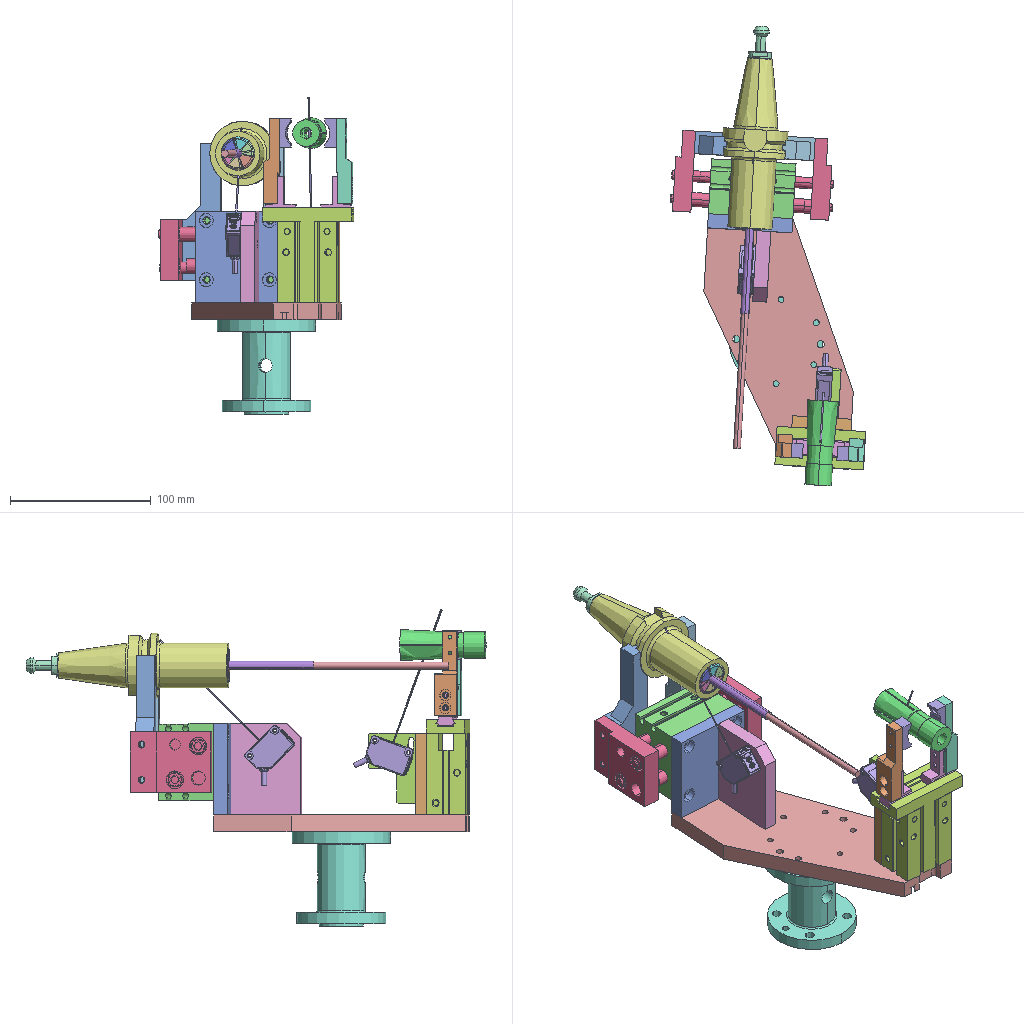Assembly | SolidWorks | 26 different items | 31 placed | box 139 x 326 x 225 mm
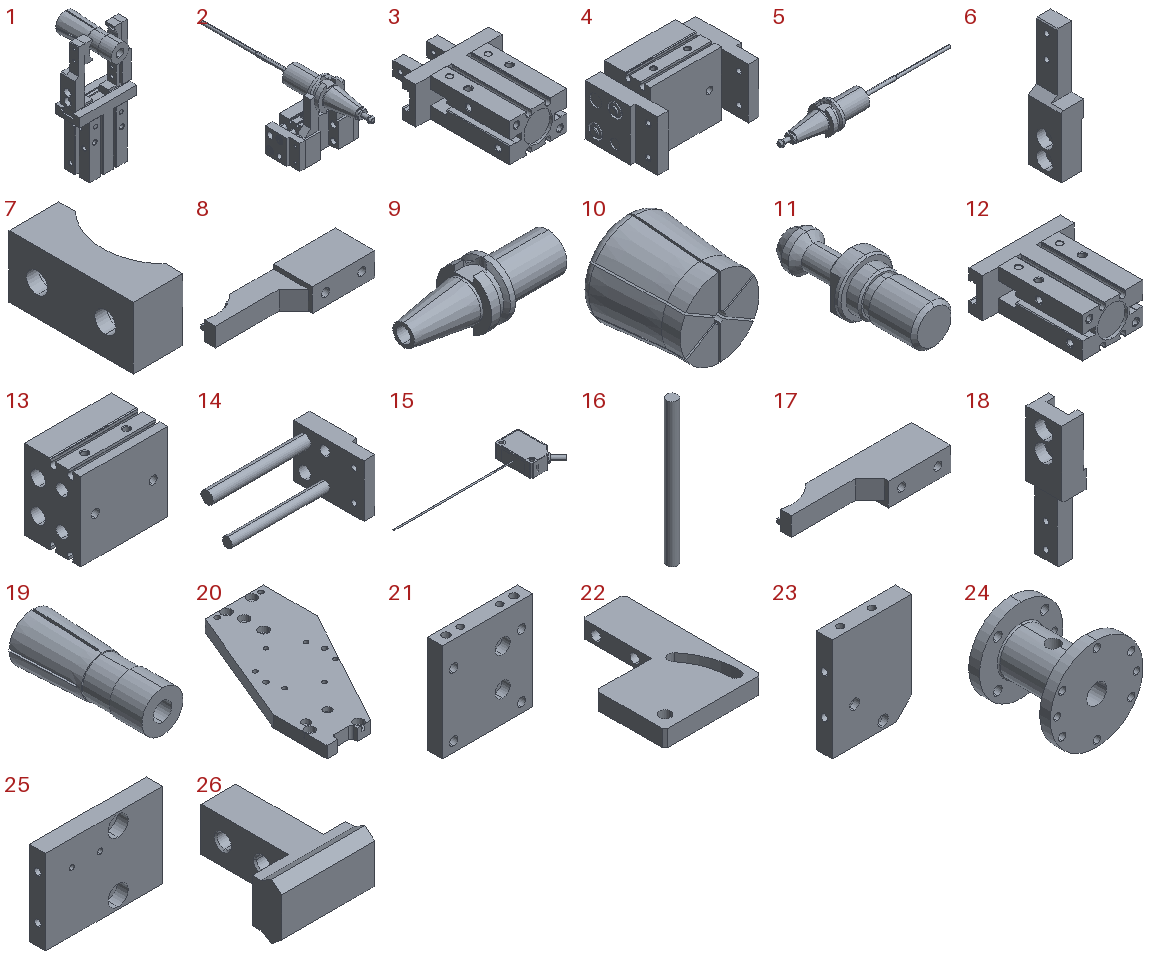Parts list (item | name | quantity | parent item | size | volume | features):
1 | (subassembly) | x1 | - | 63 x 60 x 131.489 mm | 99433 mm3 | features ReferencePattern 2, MirrorCompFeat 1
2 | (subassembly) | x1 | - | 115 x 300 x 119 mm | 333803 mm3 | features MirrorCompFeat 1, ReferencePattern 1
3 | (subassembly) | x1 | in 1 | 63 x 90 x 27.5 mm | 71296 mm3 | -
4 | (subassembly) | x1 | in 2 | 98 x 58 x 55 mm | 176822 mm3 | -
5 | (subassembly) | x1 | in 2 | 300 x 46 x 46 mm | 105904 mm3 | -
6 | - | x1 | in 1 | 11 x 16 x 60 mm | 5664 mm3 | features ICE 7, Chamfer 2, Fillet 2, HoleWzd 2, Cut 1, Extrusion 1
7 | - | x2 | in 1 | 8 x 20 x 10 mm | 974.548 mm3 | features Extrusion 1, HoleWzd 1, RevCut 1
8 | - | x1 | in 2 | 97 x 27 x 16 mm | 25539 mm3 | features ICE 9, Chamfer 2, Cut 1, Extrusion 1, Fillet 1, HoleWzd 1, MirrorPattern 1, RefAxis 1
9 | - | x1 | in 5 | 120.4 x 46 x 46 mm | 69900 mm3 | features ICE 5, Fillet 1, MirrorPattern 1, RefAxis 1, Revolution 1
10 | - | x1 | in 5 | 24.134 x 25 x 24.129 mm | 8899 mm3 | features ICE 4, RefAxis 1, Revolution 1
11 | - | x1 | in 5 | 16.4 x 43 x 16.4 mm | 4091 mm3 | features Chamfer 2, ICE 1, Revolution 1
12 | - | x1 | in 3 | 63 x 67.6 x 27.5 mm | 65251 mm3 | features BaseBody 1
13 | - | x1 | in 4 | 60 x 39 x 55 mm | 104466 mm3 | features BaseBody 1
14 | - | x2 | in 4 | 95 x 57.5 x 43 mm | 36178 mm3 | features BaseBody 1
15 | - | x2 | - | 126.19 x 38.39 x 11 mm | 6688 mm3 | features BaseBody 1, ICE 1
16 | - | x1 | in 5 | 6 x 6 x 80 mm | 2262 mm3 | features Extrusion 1
17 | - | x1 | in 2 | 97 x 27 x 16 mm | 25539 mm3 | features MirrorStock 1
18 | - | x1 | in 1 | 11 x 16 x 60 mm | 5664 mm3 | features MirrorStock 1
19 | - | x2 | in 1, 5 | 21.977 x 60 x 21.977 mm | 14861 mm3 | features ICE 3, 3DProfileFeature 1, HoleWzd 1, Revolution 1
20 | - | x1 | - | 110 x 175 x 12 mm | 140751 mm3 | features HoleWzd 7, Chamfer 2, Extrusion 1, Fillet 1, ICE 1, RefAxis 1
21 | - | x1 | - | 60 x 10 x 65 mm | 35169 mm3 | features HoleWzd 4, Extrusion 1
22 | - | x1 | - | 35 x 50 x 6 mm | 6636 mm3 | features Chamfer 1, Cut 1, Extrusion 1, HoleWzd 1, ICE 1
23 | - | x1 | - | 50 x 10 x 65 mm | 30944 mm3 | features HoleWzd 3, Chamfer 2, Extrusion 1, ICE 1
24 | - | x1 | - | 70 x 67 x 70 mm | 85773 mm3 | features ICE 5, HoleWzd 2, Cut 1, Extrusion 1, Fillet 1, Helix 1, RevCut 1
25 | - | x1 | - | 58 x 8 x 42 mm | 18259 mm3 | features HoleWzd 3, Extrusion 1
26 | - | x2 | in 3 | 21.4 x 26.74 x 12.8 mm | 3023 mm3 | features BaseBody 1
Mates (type | each side: item.copy, entity, surface, feature):
In the top assembly
Coincident | 20.1 face plane Boss-Extrude 1 | 21.1 face plane Boss-Extrude 1 | 3 times
Concentric | 21.1 face cylinder M5 六角凹头Screw的柱形沉头Hole 2 | 23.1 face cylinder M5 Tapped Hole 1
Coincident | 21.1 face plane Boss-Extrude 1 | 23.1 face plane Boss-Extrude 1
Parallel | 21.1 face plane Boss-Extrude 1 | 23.1 face plane Boss-Extrude 1
Coincident | 20.1 face plane Boss-Extrude 1 | 24.1 face plane Boss-Extrude 1
Concentric | 23.1 face cylinder M3 六角凹头Screw的柱形沉头Hole 1 | 15.1 face cylinder E-MSMD61N-2M_l-1-solid1 | 2 times
Coincident | 23.1 face plane Boss-Extrude 1 | 15.1 face plane E-MSMD61N-2M_l-1-solid1
Coincident | 20.1 face plane Boss-Extrude 1 | 25.1 face plane Boss-Extrude 1
Coincident | 25.1 face plane Boss-Extrude 1 | 22.1 face plane Boss-Extrude 1 | 2 times
Coincident | 15.2 face plane E-MSMD61N-2M_l-1-solid1 | 22.1 face plane Boss-Extrude 1
Concentric | 15.2 face cylinder E-MSMD61N-2M_l-1-solid1 | 22.1 face cylinder Cut-Extrude 2
PlanarAngleDim | 15.2 face plane E-MSMD61N-2M_l-1-solid1 | 22.1 face plane Boss-Extrude 1
Symmetric | 25.1 face plane Boss-Extrude 1 | 25.1 face plane Boss-Extrude 1 | 15.2 plane
Concentric | 20.1 axis | 24.1 face cylinder Cut-Revolve 1
Concentric | 20.1 face cylinder Ø5.0mm 暗销Hole 1 | 24.1 face cylinder Ø5.0mm 暗销Hole 1
Coincident | 21.1 face plane Boss-Extrude 1 | 13.1 face plane 输入1
Concentric | 21.1 face cylinder M5 六角凹头Screw的柱形沉头Hole 1 | 13.1 face cylinder 输入1 | 2 times
Coincident | 20.1 face plane Boss-Extrude 1 | 12.1 face plane 输入1
Concentric | 20.1 face cylinder M5 六角凹头Screw的柱形沉头Hole 6 | 12.1 face cylinder 输入1 | 2 times
In subassembly 1
Coincident | 3.1 plane | 1.1 plane | 3 times
Coincident | 26.1 face plane 输入1 | 6.1 face plane Cut-Extrude 1 | 2 times
Width | 6.1 face plane Boss-Extrude 1 | 6.1 face plane Boss-Extrude 1 | 26.1 face plane 输入1 | 26.1 face plane 输入1
DistanceDim | 19.1 face plane Revolve 1 | 6.1 face plane Boss-Extrude 1
DistanceDim | 19.1 plane | 6.1 face plane Boss-Extrude 1
Symmetric | 12.2 face plane 输入1 | 12.2 face plane 输入1 | 19.1 plane
Coincident | 6.1 face plane Cut-Extrude 10 | 7.1 face plane Boss-Extrude 1
Concentric | 6.1 face cylinder M3 Tapped Hole 1 | 7.1 face cylinder M3 六角圆柱头Screw的柱形沉头Hole 1 | 2 times
In subassembly 3
Width | 12.3 face plane 输入1 | 12.3 face plane 输入1 | 26.2 face plane 输入1 | 26.2 face plane 输入1
DistanceDim | 26.2 face plane 输入1 | 12.3 face plane 输入1
Coincident | 26.3 face plane 输入1 | 26.2 face plane 输入1 | 2 times
LimitDistanceDim | 26.3 face plane 输入1 | 26.2 face plane 输入1
Width | 12.3 face plane 输入1 | 12.3 face plane 输入1 | 26.3 face plane 输入1 | 26.2 face plane 输入1
In subassembly 2
Coincident | 4.1 plane | 5.1 plane
Symmetric | 8.1 face plane Cut-Extrude 4 | 8.1 face plane Cut-Extrude 3 | 9.1 plane
Coincident | 14.1 face plane 输入1 | 8.1 face plane Boss-Extrude 1 | 3 times
Concentric | 8.1 face cylinder Cut-Extrude 4 | 9.1 face cylinder Boss-Extrude 1
In subassembly 5
Coincident | 9.2 plane | 5.2 plane | 3 times
Concentric | 9.2 face cylinder Cut-Extrude 2 | 11.1 face cylinder Revolve 1
Coincident | 9.2 face plane Revolve 1 | 11.1 face plane Revolve 1
Coincident | 9.2 plane | 11.1 plane
Concentric | 9.2 face cylinder Cut-Extrude 3 | 10.1 face cylinder Revolve 1
DistanceDim | 10.1 face plane Revolve 1 | 9.2 face plane Boss-Extrude 1
Concentric | 10.1 face cylinder Cut-Extrude 1 | 16.1 face cylinder Boss-Extrude 1
DistanceDim | 16.1 face plane Boss-Extrude 1 | 10.1 face plane Revolve 1
Concentric | 9.2 face cylinder Cut-Extrude 3 | 19.1 face cylinder Revolve 1
Coincident | 9.2 face plane Boss-Extrude 1 | 19.1 face plane Revolve 1
In subassembly 4
LimitDistanceDim | 14.2 face plane 输入1 | 14.3 face plane 输入1
Width | 14.3 face plane 输入1 | 14.2 face plane 输入1 | 13.2 face plane 输入1 | 13.2 face plane 输入1
Concentric | 13.2 face cylinder 输入1 | 14.3 face cylinder 输入1
Parallel | 13.2 face plane 输入1 | 14.3 face plane 输入1
Concentric | 13.2 face cylinder 输入1 | 14.2 face cylinder 输入1
Parallel | 14.3 face plane 输入1 | 14.2 face plane 输入1